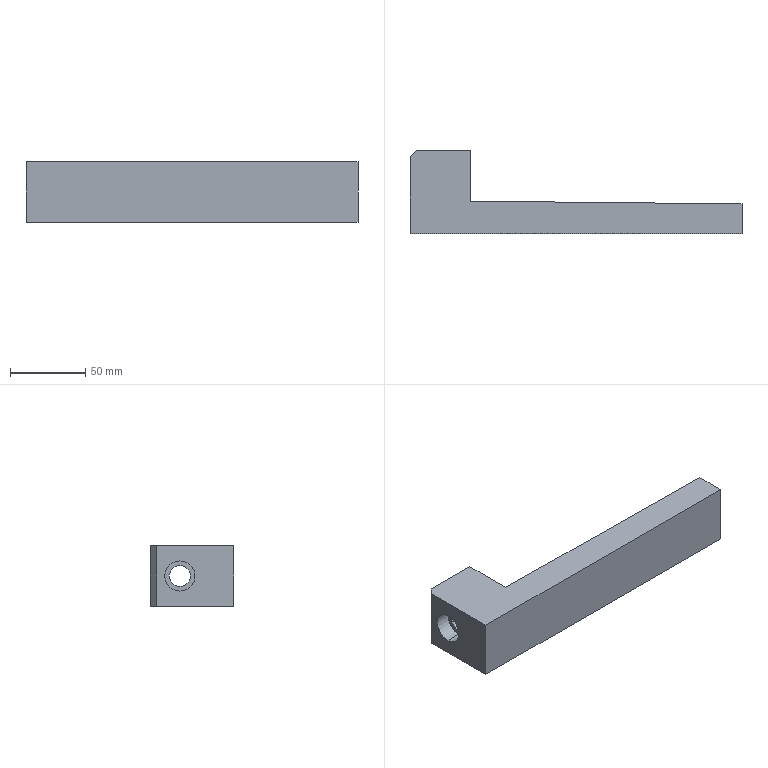Part | NX | features BREP 1 | 1 solid | 14 faces | box 220 x 55 x 40 mm | volume 227539 mm3 | plane 10 | cylinder 4 | commonest cylinder face diameters 14 x2 20 x2
STEP:
#1=CARTESIAN_POINT('',(-200.,35.5,-7.));
#2=VERTEX_POINT('',#1);
#3=CARTESIAN_POINT('',(-200.,35.5,7.));
#4=VERTEX_POINT('',#3);
#5=CARTESIAN_POINT('',(-200.,35.5,0.));
#6=DIRECTION('',(-1.,0.,0.));
#7=DIRECTION('',(0.,0.,1.));
#8=AXIS2_PLACEMENT_3D('',#5,#6,#7);
#9=CIRCLE('',#8,7.);
#10=EDGE_CURVE('',#2,#4,#9,.T.);
#11=ORIENTED_EDGE('',*,*,#10,.F.);
#12=CARTESIAN_POINT('',(-230.,35.5,-7.));
#13=VERTEX_POINT('',#12);
#14=CARTESIAN_POINT('',(0.,35.5,-7.));
#15=DIRECTION('',(-1.,0.,0.));
#16=VECTOR('',#15,1000.);
#17=LINE('',#14,#16);
#18=EDGE_CURVE('',#2,#13,#17,.T.);
#19=ORIENTED_EDGE('',*,*,#18,.T.);
#20=CARTESIAN_POINT('',(-230.,35.5,7.));
#21=VERTEX_POINT('',#20);
#22=CARTESIAN_POINT('',(-230.,35.5,0.));
#23=DIRECTION('',(-1.,0.,0.));
#24=DIRECTION('',(0.,0.,1.));
#25=AXIS2_PLACEMENT_3D('',#22,#23,#24);
#26=CIRCLE('',#25,7.);
#27=EDGE_CURVE('',#13,#21,#26,.T.);
#28=ORIENTED_EDGE('',*,*,#27,.T.);
#29=CARTESIAN_POINT('',(0.,35.5,7.));
#30=DIRECTION('',(-1.,0.,0.));
#31=VECTOR('',#30,1000.);
#32=LINE('',#29,#31);
#33=EDGE_CURVE('',#4,#21,#32,.T.);
#34=ORIENTED_EDGE('',*,*,#33,.F.);
#35=EDGE_LOOP('',(#11,#19,#28,#34));
#36=FACE_BOUND('',#35,.T.);
#37=CARTESIAN_POINT('',(0.,35.5,0.));
#38=DIRECTION('',(-1.,0.,0.));
#39=DIRECTION('',(0.,0.,-1.));
#40=AXIS2_PLACEMENT_3D('',#37,#38,#39);
#41=CYLINDRICAL_SURFACE('',#40,7.);
#42=ADVANCED_FACE('',(#36),#41,.F.);
#43=CARTESIAN_POINT('',(-230.,35.5,-10.));
#44=VERTEX_POINT('',#43);
#45=CARTESIAN_POINT('',(-230.,35.5,10.));
#46=VERTEX_POINT('',#45);
#47=CARTESIAN_POINT('',(-230.,35.5,0.));
#48=DIRECTION('',(-1.,0.,0.));
#49=DIRECTION('',(0.,0.,1.));
#50=AXIS2_PLACEMENT_3D('',#47,#48,#49);
#51=CIRCLE('',#50,10.);
#52=EDGE_CURVE('',#44,#46,#51,.T.);
#53=ORIENTED_EDGE('',*,*,#52,.F.);
#54=CARTESIAN_POINT('',(-240.,35.5,-10.));
#55=VERTEX_POINT('',#54);
#56=CARTESIAN_POINT('',(-230.,35.5,-10.));
#57=DIRECTION('',(-1.,0.,0.));
#58=VECTOR('',#57,1000.);
#59=LINE('',#56,#58);
#60=EDGE_CURVE('',#44,#55,#59,.T.);
#61=ORIENTED_EDGE('',*,*,#60,.T.);
#62=CARTESIAN_POINT('',(-240.,35.5,10.));
#63=VERTEX_POINT('',#62);
#64=CARTESIAN_POINT('',(-240.,35.5,0.));
#65=DIRECTION('',(-1.,0.,0.));
#66=DIRECTION('',(0.,0.,1.));
#67=AXIS2_PLACEMENT_3D('',#64,#65,#66);
#68=CIRCLE('',#67,10.);
#69=EDGE_CURVE('',#55,#63,#68,.T.);
#70=ORIENTED_EDGE('',*,*,#69,.T.);
#71=CARTESIAN_POINT('',(-230.,35.5,10.));
#72=DIRECTION('',(-1.,0.,0.));
#73=VECTOR('',#72,1000.);
#74=LINE('',#71,#73);
#75=EDGE_CURVE('',#46,#63,#74,.T.);
#76=ORIENTED_EDGE('',*,*,#75,.F.);
#77=EDGE_LOOP('',(#53,#61,#70,#76));
#78=FACE_BOUND('',#77,.T.);
#79=CARTESIAN_POINT('',(-230.,35.5,0.));
#80=DIRECTION('',(-1.,0.,0.));
#81=DIRECTION('',(0.,0.,-1.));
#82=AXIS2_PLACEMENT_3D('',#79,#80,#81);
#83=CYLINDRICAL_SURFACE('',#82,10.);
#84=ADVANCED_FACE('',(#78),#83,.F.);
#85=CARTESIAN_POINT('',(-20.,19.607,20.));
#86=VERTEX_POINT('',#85);
#87=CARTESIAN_POINT('',(-200.,21.398,20.));
#88=VERTEX_POINT('',#87);
#89=CARTESIAN_POINT('',(-200.,21.398,20.));
#90=DIRECTION('',(-1.,0.009948,0.));
#91=VECTOR('',#90,1000.);
#92=LINE('',#89,#91);
#93=EDGE_CURVE('',#86,#88,#92,.T.);
#94=ORIENTED_EDGE('',*,*,#93,.F.);
#95=CARTESIAN_POINT('',(-20.,19.607,-20.));
#96=VERTEX_POINT('',#95);
#97=CARTESIAN_POINT('',(-20.,19.607,20.));
#98=DIRECTION('',(0.,0.,-1.));
#99=VECTOR('',#98,1000.);
#100=LINE('',#97,#99);
#101=EDGE_CURVE('',#86,#96,#100,.T.);
#102=ORIENTED_EDGE('',*,*,#101,.T.);
#103=CARTESIAN_POINT('',(-200.,21.398,-20.));
#104=VERTEX_POINT('',#103);
#105=CARTESIAN_POINT('',(-200.,21.398,-20.));
#106=DIRECTION('',(-1.,0.009948,0.));
#107=VECTOR('',#106,1000.);
#108=LINE('',#105,#107);
#109=EDGE_CURVE('',#96,#104,#108,.T.);
#110=ORIENTED_EDGE('',*,*,#109,.T.);
#111=CARTESIAN_POINT('',(-200.,21.398,20.));
#112=DIRECTION('',(0.,0.,-1.));
#113=VECTOR('',#112,1000.);
#114=LINE('',#111,#113);
#115=EDGE_CURVE('',#88,#104,#114,.T.);
#116=ORIENTED_EDGE('',*,*,#115,.F.);
#117=EDGE_LOOP('',(#94,#102,#110,#116));
#118=FACE_BOUND('',#117,.T.);
#119=CARTESIAN_POINT('',(-200.,21.398,20.));
#120=DIRECTION('',(-0.009948,-1.,0.));
#121=DIRECTION('',(-1.,0.009948,0.));
#122=AXIS2_PLACEMENT_3D('',#119,#120,#121);
#123=PLANE('',#122);
#124=ADVANCED_FACE('',(#118),#123,.F.);
#125=CARTESIAN_POINT('',(-200.,35.5,0.));
#126=DIRECTION('',(-1.,0.,0.));
#127=DIRECTION('',(0.,0.,1.));
#128=AXIS2_PLACEMENT_3D('',#125,#126,#127);
#129=CIRCLE('',#128,7.);
#130=EDGE_CURVE('',#4,#2,#129,.T.);
#131=ORIENTED_EDGE('',*,*,#130,.T.);
#132=ORIENTED_EDGE('',*,*,#10,.T.);
#133=EDGE_LOOP('',(#131,#132));
#134=FACE_BOUND('',#133,.T.);
#135=CARTESIAN_POINT('',(-200.,55.,-20.));
#136=VERTEX_POINT('',#135);
#137=CARTESIAN_POINT('',(-200.,55.,-20.));
#138=DIRECTION('',(0.,1.,0.));
#139=VECTOR('',#138,1000.);
#140=LINE('',#137,#139);
#141=EDGE_CURVE('',#104,#136,#140,.T.);
#142=ORIENTED_EDGE('',*,*,#141,.T.);
#143=CARTESIAN_POINT('',(-200.,55.,20.));
#144=VERTEX_POINT('',#143);
#145=CARTESIAN_POINT('',(-200.,55.,20.));
#146=DIRECTION('',(0.,0.,-1.));
#147=VECTOR('',#146,1000.);
#148=LINE('',#145,#147);
#149=EDGE_CURVE('',#144,#136,#148,.T.);
#150=ORIENTED_EDGE('',*,*,#149,.F.);
#151=CARTESIAN_POINT('',(-200.,55.,20.));
#152=DIRECTION('',(0.,1.,0.));
#153=VECTOR('',#152,1000.);
#154=LINE('',#151,#153);
#155=EDGE_CURVE('',#88,#144,#154,.T.);
#156=ORIENTED_EDGE('',*,*,#155,.F.);
#157=ORIENTED_EDGE('',*,*,#115,.T.);
#158=EDGE_LOOP('',(#142,#150,#156,#157));
#159=FACE_BOUND('',#158,.T.);
#160=CARTESIAN_POINT('',(-200.,55.,20.));
#161=DIRECTION('',(-1.,0.,0.));
#162=DIRECTION('',(0.,0.,-1.));
#163=AXIS2_PLACEMENT_3D('',#160,#161,#162);
#164=PLANE('',#163);
#165=ADVANCED_FACE('',(#134,#159),#164,.F.);
#166=CARTESIAN_POINT('',(-236.,55.,-20.));
#167=VERTEX_POINT('',#166);
#168=CARTESIAN_POINT('',(-236.,55.,-20.));
#169=DIRECTION('',(-1.,0.,0.));
#170=VECTOR('',#169,1000.);
#171=LINE('',#168,#170);
#172=EDGE_CURVE('',#136,#167,#171,.T.);
#173=ORIENTED_EDGE('',*,*,#172,.T.);
#174=CARTESIAN_POINT('',(-236.,55.,20.));
#175=VERTEX_POINT('',#174);
#176=CARTESIAN_POINT('',(-236.,55.,20.));
#177=DIRECTION('',(0.,0.,-1.));
#178=VECTOR('',#177,1000.);
#179=LINE('',#176,#178);
#180=EDGE_CURVE('',#175,#167,#179,.T.);
#181=ORIENTED_EDGE('',*,*,#180,.F.);
#182=CARTESIAN_POINT('',(-236.,55.,20.));
#183=DIRECTION('',(-1.,0.,0.));
#184=VECTOR('',#183,1000.);
#185=LINE('',#182,#184);
#186=EDGE_CURVE('',#144,#175,#185,.T.);
#187=ORIENTED_EDGE('',*,*,#186,.F.);
#188=ORIENTED_EDGE('',*,*,#149,.T.);
#189=EDGE_LOOP('',(#173,#181,#187,#188));
#190=FACE_BOUND('',#189,.T.);
#191=CARTESIAN_POINT('',(-236.,55.,20.));
#192=DIRECTION('',(0.,-1.,0.));
#193=DIRECTION('',(0.,0.,1.));
#194=AXIS2_PLACEMENT_3D('',#191,#192,#193);
#195=PLANE('',#194);
#196=ADVANCED_FACE('',(#190),#195,.F.);
#197=CARTESIAN_POINT('',(-240.,51.,-20.));
#198=VERTEX_POINT('',#197);
#199=CARTESIAN_POINT('',(-240.,51.,-20.));
#200=DIRECTION('',(-0.7071,-0.7071,0.));
#201=VECTOR('',#200,1000.);
#202=LINE('',#199,#201);
#203=EDGE_CURVE('',#167,#198,#202,.T.);
#204=ORIENTED_EDGE('',*,*,#203,.T.);
#205=CARTESIAN_POINT('',(-240.,51.,20.));
#206=VERTEX_POINT('',#205);
#207=CARTESIAN_POINT('',(-240.,51.,20.));
#208=DIRECTION('',(0.,0.,-1.));
#209=VECTOR('',#208,1000.);
#210=LINE('',#207,#209);
#211=EDGE_CURVE('',#206,#198,#210,.T.);
#212=ORIENTED_EDGE('',*,*,#211,.F.);
#213=CARTESIAN_POINT('',(-240.,51.,20.));
#214=DIRECTION('',(-0.7071,-0.7071,0.));
#215=VECTOR('',#214,1000.);
#216=LINE('',#213,#215);
#217=EDGE_CURVE('',#175,#206,#216,.T.);
#218=ORIENTED_EDGE('',*,*,#217,.F.);
#219=ORIENTED_EDGE('',*,*,#180,.T.);
#220=EDGE_LOOP('',(#204,#212,#218,#219));
#221=FACE_BOUND('',#220,.T.);
#222=CARTESIAN_POINT('',(-240.,51.,20.));
#223=DIRECTION('',(0.7071,-0.7071,0.));
#224=DIRECTION('',(-0.7071,-0.7071,0.));
#225=AXIS2_PLACEMENT_3D('',#222,#223,#224);
#226=PLANE('',#225);
#227=ADVANCED_FACE('',(#221),#226,.F.);
#228=CARTESIAN_POINT('',(-240.,35.5,0.));
#229=DIRECTION('',(-1.,0.,0.));
#230=DIRECTION('',(0.,0.,1.));
#231=AXIS2_PLACEMENT_3D('',#228,#229,#230);
#232=CIRCLE('',#231,10.);
#233=EDGE_CURVE('',#63,#55,#232,.T.);
#234=ORIENTED_EDGE('',*,*,#233,.F.);
#235=ORIENTED_EDGE('',*,*,#69,.F.);
#236=EDGE_LOOP('',(#234,#235));
#237=FACE_BOUND('',#236,.T.);
#238=CARTESIAN_POINT('',(-240.,0.,-20.));
#239=VERTEX_POINT('',#238);
#240=CARTESIAN_POINT('',(-240.,0.,-20.));
#241=DIRECTION('',(0.,-1.,0.));
#242=VECTOR('',#241,1000.);
#243=LINE('',#240,#242);
#244=EDGE_CURVE('',#198,#239,#243,.T.);
#245=ORIENTED_EDGE('',*,*,#244,.T.);
#246=CARTESIAN_POINT('',(-240.,0.,20.));
#247=VERTEX_POINT('',#246);
#248=CARTESIAN_POINT('',(-240.,0.,20.));
#249=DIRECTION('',(0.,0.,-1.));
#250=VECTOR('',#249,1000.);
#251=LINE('',#248,#250);
#252=EDGE_CURVE('',#247,#239,#251,.T.);
#253=ORIENTED_EDGE('',*,*,#252,.F.);
#254=CARTESIAN_POINT('',(-240.,0.,20.));
#255=DIRECTION('',(0.,-1.,0.));
#256=VECTOR('',#255,1000.);
#257=LINE('',#254,#256);
#258=EDGE_CURVE('',#206,#247,#257,.T.);
#259=ORIENTED_EDGE('',*,*,#258,.F.);
#260=ORIENTED_EDGE('',*,*,#211,.T.);
#261=EDGE_LOOP('',(#245,#253,#259,#260));
#262=FACE_BOUND('',#261,.T.);
#263=CARTESIAN_POINT('',(-240.,0.,20.));
#264=DIRECTION('',(1.,0.,0.));
#265=DIRECTION('',(0.,0.,1.));
#266=AXIS2_PLACEMENT_3D('',#263,#264,#265);
#267=PLANE('',#266);
#268=ADVANCED_FACE('',(#237,#262),#267,.F.);
#269=CARTESIAN_POINT('',(-20.,0.,-20.));
#270=VERTEX_POINT('',#269);
#271=CARTESIAN_POINT('',(0.,0.,-20.));
#272=DIRECTION('',(1.,0.,0.));
#273=VECTOR('',#272,1000.);
#274=LINE('',#271,#273);
#275=EDGE_CURVE('',#239,#270,#274,.T.);
#276=ORIENTED_EDGE('',*,*,#275,.T.);
#277=CARTESIAN_POINT('',(-20.,0.,20.));
#278=VERTEX_POINT('',#277);
#279=CARTESIAN_POINT('',(-20.,0.,20.));
#280=DIRECTION('',(0.,0.,1.));
#281=VECTOR('',#280,1000.);
#282=LINE('',#279,#281);
#283=EDGE_CURVE('',#270,#278,#282,.T.);
#284=ORIENTED_EDGE('',*,*,#283,.T.);
#285=CARTESIAN_POINT('',(0.,0.,20.));
#286=DIRECTION('',(1.,0.,0.));
#287=VECTOR('',#286,1000.);
#288=LINE('',#285,#287);
#289=EDGE_CURVE('',#247,#278,#288,.T.);
#290=ORIENTED_EDGE('',*,*,#289,.F.);
#291=ORIENTED_EDGE('',*,*,#252,.T.);
#292=EDGE_LOOP('',(#276,#284,#290,#291));
#293=FACE_BOUND('',#292,.T.);
#294=CARTESIAN_POINT('',(0.,0.,20.));
#295=DIRECTION('',(0.,1.,0.));
#296=DIRECTION('',(1.,0.,0.));
#297=AXIS2_PLACEMENT_3D('',#294,#295,#296);
#298=PLANE('',#297);
#299=ADVANCED_FACE('',(#293),#298,.F.);
#300=CARTESIAN_POINT('',(-20.,68.818,20.));
#301=DIRECTION('',(0.,-1.,0.));
#302=VECTOR('',#301,1000.);
#303=LINE('',#300,#302);
#304=EDGE_CURVE('',#86,#278,#303,.T.);
#305=ORIENTED_EDGE('',*,*,#304,.F.);
#306=ORIENTED_EDGE('',*,*,#93,.T.);
#307=ORIENTED_EDGE('',*,*,#155,.T.);
#308=ORIENTED_EDGE('',*,*,#186,.T.);
#309=ORIENTED_EDGE('',*,*,#217,.T.);
#310=ORIENTED_EDGE('',*,*,#258,.T.);
#311=ORIENTED_EDGE('',*,*,#289,.T.);
#312=EDGE_LOOP('',(#305,#306,#307,#308,#309,#310,#311));
#313=FACE_BOUND('',#312,.T.);
#314=CARTESIAN_POINT('',(0.,55.,20.));
#315=DIRECTION('',(0.,0.,1.));
#316=DIRECTION('',(-1.,0.,0.));
#317=AXIS2_PLACEMENT_3D('',#314,#315,#316);
#318=PLANE('',#317);
#319=ADVANCED_FACE('',(#313),#318,.T.);
#320=ORIENTED_EDGE('',*,*,#109,.F.);
#321=CARTESIAN_POINT('',(-20.,55.,-20.));
#322=DIRECTION('',(0.,-1.,0.));
#323=VECTOR('',#322,1000.);
#324=LINE('',#321,#323);
#325=EDGE_CURVE('',#96,#270,#324,.T.);
#326=ORIENTED_EDGE('',*,*,#325,.T.);
#327=ORIENTED_EDGE('',*,*,#275,.F.);
#328=ORIENTED_EDGE('',*,*,#244,.F.);
#329=ORIENTED_EDGE('',*,*,#203,.F.);
#330=ORIENTED_EDGE('',*,*,#172,.F.);
#331=ORIENTED_EDGE('',*,*,#141,.F.);
#332=EDGE_LOOP('',(#320,#326,#327,#328,#329,#330,#331));
#333=FACE_BOUND('',#332,.T.);
#334=CARTESIAN_POINT('',(0.,55.,-20.));
#335=DIRECTION('',(0.,0.,1.));
#336=DIRECTION('',(-1.,0.,0.));
#337=AXIS2_PLACEMENT_3D('',#334,#335,#336);
#338=PLANE('',#337);
#339=ADVANCED_FACE('',(#333),#338,.F.);
#340=ORIENTED_EDGE('',*,*,#60,.F.);
#341=CARTESIAN_POINT('',(-230.,35.5,0.));
#342=DIRECTION('',(-1.,0.,0.));
#343=DIRECTION('',(0.,0.,1.));
#344=AXIS2_PLACEMENT_3D('',#341,#342,#343);
#345=CIRCLE('',#344,10.);
#346=EDGE_CURVE('',#46,#44,#345,.T.);
#347=ORIENTED_EDGE('',*,*,#346,.F.);
#348=ORIENTED_EDGE('',*,*,#75,.T.);
#349=ORIENTED_EDGE('',*,*,#233,.T.);
#350=EDGE_LOOP('',(#340,#347,#348,#349));
#351=FACE_BOUND('',#350,.T.);
#352=CARTESIAN_POINT('',(-230.,35.5,0.));
#353=DIRECTION('',(-1.,0.,0.));
#354=DIRECTION('',(0.,0.,-1.));
#355=AXIS2_PLACEMENT_3D('',#352,#353,#354);
#356=CYLINDRICAL_SURFACE('',#355,10.);
#357=ADVANCED_FACE('',(#351),#356,.F.);
#358=CARTESIAN_POINT('',(-230.,35.5,0.));
#359=DIRECTION('',(-1.,0.,0.));
#360=DIRECTION('',(0.,0.,1.));
#361=AXIS2_PLACEMENT_3D('',#358,#359,#360);
#362=CIRCLE('',#361,7.);
#363=EDGE_CURVE('',#21,#13,#362,.T.);
#364=ORIENTED_EDGE('',*,*,#363,.F.);
#365=ORIENTED_EDGE('',*,*,#27,.F.);
#366=EDGE_LOOP('',(#364,#365));
#367=FACE_BOUND('',#366,.T.);
#368=ORIENTED_EDGE('',*,*,#346,.T.);
#369=ORIENTED_EDGE('',*,*,#52,.T.);
#370=EDGE_LOOP('',(#368,#369));
#371=FACE_BOUND('',#370,.T.);
#372=CARTESIAN_POINT('',(-230.,35.5,0.));
#373=DIRECTION('',(-1.,0.,0.));
#374=DIRECTION('',(0.,0.,-1.));
#375=AXIS2_PLACEMENT_3D('',#372,#373,#374);
#376=PLANE('',#375);
#377=ADVANCED_FACE('',(#367,#371),#376,.T.);
#378=ORIENTED_EDGE('',*,*,#18,.F.);
#379=ORIENTED_EDGE('',*,*,#130,.F.);
#380=ORIENTED_EDGE('',*,*,#33,.T.);
#381=ORIENTED_EDGE('',*,*,#363,.T.);
#382=EDGE_LOOP('',(#378,#379,#380,#381));
#383=FACE_BOUND('',#382,.T.);
#384=CARTESIAN_POINT('',(0.,35.5,0.));
#385=DIRECTION('',(-1.,0.,0.));
#386=DIRECTION('',(0.,0.,-1.));
#387=AXIS2_PLACEMENT_3D('',#384,#385,#386);
#388=CYLINDRICAL_SURFACE('',#387,7.);
#389=ADVANCED_FACE('',(#383),#388,.F.);
#390=ORIENTED_EDGE('',*,*,#304,.T.);
#391=ORIENTED_EDGE('',*,*,#283,.F.);
#392=ORIENTED_EDGE('',*,*,#325,.F.);
#393=ORIENTED_EDGE('',*,*,#101,.F.);
#394=EDGE_LOOP('',(#390,#391,#392,#393));
#395=FACE_BOUND('',#394,.T.);
#396=CARTESIAN_POINT('',(-20.,68.818,-20.));
#397=DIRECTION('',(-1.,0.,0.));
#398=DIRECTION('',(0.,1.,0.));
#399=AXIS2_PLACEMENT_3D('',#396,#397,#398);
#400=PLANE('',#399);
#401=ADVANCED_FACE('',(#395),#400,.F.);
#402=CLOSED_SHELL('',(#42,#84,#124,#165,#196,#227,#268,#299,#319,#339,#357,#377,#389,#401));
#403=MANIFOLD_SOLID_BREP('',#402);
#404=(LENGTH_UNIT()NAMED_UNIT(*)SI_UNIT(.MILLI.,.METRE.));
#405=UNCERTAINTY_MEASURE_WITH_UNIT(LENGTH_MEASURE(0.00001),#404,'','');
#406=(NAMED_UNIT(*)PLANE_ANGLE_UNIT()SI_UNIT($,.RADIAN.));
#407=(NAMED_UNIT(*)SI_UNIT($,.STERADIAN.)SOLID_ANGLE_UNIT());
#408=(GEOMETRIC_REPRESENTATION_CONTEXT(3)GLOBAL_UNCERTAINTY_ASSIGNED_CONTEXT((#405))GLOBAL_UNIT_ASSIGNED_CONTEXT((#404,#406,#407))REPRESENTATION_CONTEXT('',''));
#409=ADVANCED_BREP_SHAPE_REPRESENTATION('',(#403),#408);